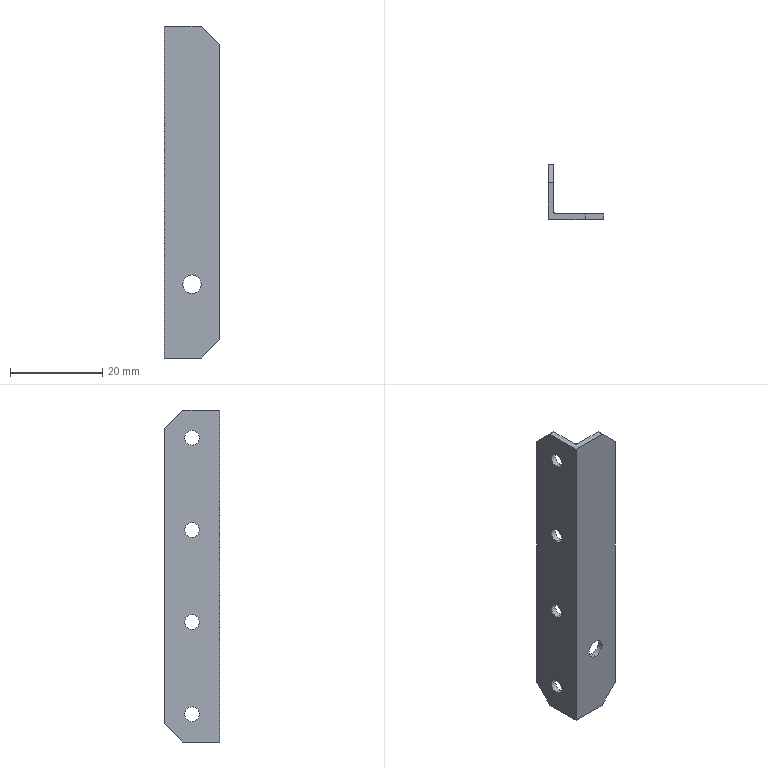Part | SolidWorks | features BaseBody 1 | 1 solid | 23 faces | box 12 x 12 x 72 mm | volume 1882 mm3 | plane 12 | cylinder 11 | commonest cylinder face diameters 3.2 x8 4 x2 1 x1
STEP:
#1=CARTESIAN_POINT('',(6.,0.,18.));
#2=VERTEX_POINT('',#1);
#3=CARTESIAN_POINT('',(6.,0.,14.));
#4=VERTEX_POINT('',#3);
#5=CARTESIAN_POINT('',(6.,0.,16.));
#6=DIRECTION('',(0.,-1.,0.));
#7=DIRECTION('',(0.,0.,1.));
#8=AXIS2_PLACEMENT_3D('',#5,#6,#7);
#9=CIRCLE('',#8,2.);
#10=EDGE_CURVE('',#2,#4,#9,.T.);
#11=ORIENTED_EDGE('',*,*,#10,.T.);
#12=CARTESIAN_POINT('',(6.,1.2,14.));
#13=VERTEX_POINT('',#12);
#14=CARTESIAN_POINT('',(6.,0.,14.));
#15=DIRECTION('',(0.,1.,0.));
#16=VECTOR('',#15,1000.);
#17=LINE('',#14,#16);
#18=EDGE_CURVE('',#4,#13,#17,.T.);
#19=ORIENTED_EDGE('',*,*,#18,.T.);
#20=CARTESIAN_POINT('',(6.,1.2,18.));
#21=VERTEX_POINT('',#20);
#22=CARTESIAN_POINT('',(6.,1.2,16.));
#23=DIRECTION('',(0.,1.,0.));
#24=DIRECTION('',(0.,0.,1.));
#25=AXIS2_PLACEMENT_3D('',#22,#23,#24);
#26=CIRCLE('',#25,2.);
#27=EDGE_CURVE('',#13,#21,#26,.T.);
#28=ORIENTED_EDGE('',*,*,#27,.T.);
#29=CARTESIAN_POINT('',(6.,0.,18.));
#30=DIRECTION('',(0.,1.,0.));
#31=VECTOR('',#30,1000.);
#32=LINE('',#29,#31);
#33=EDGE_CURVE('',#2,#21,#32,.T.);
#34=ORIENTED_EDGE('',*,*,#33,.F.);
#35=EDGE_LOOP('',(#11,#19,#28,#34));
#36=FACE_OUTER_BOUND('',#35,.T.);
#37=CARTESIAN_POINT('',(6.,0.,16.));
#38=DIRECTION('',(0.,1.,0.));
#39=DIRECTION('',(0.,0.,1.));
#40=AXIS2_PLACEMENT_3D('',#37,#38,#39);
#41=CYLINDRICAL_SURFACE('',#40,2.);
#42=ADVANCED_FACE('',(#36),#41,.F.);
#43=CARTESIAN_POINT('',(1.2,6.,7.6));
#44=VERTEX_POINT('',#43);
#45=CARTESIAN_POINT('',(1.2,6.,4.4));
#46=VERTEX_POINT('',#45);
#47=CARTESIAN_POINT('',(1.2,6.,6.));
#48=DIRECTION('',(1.,0.,0.));
#49=DIRECTION('',(0.,0.,1.));
#50=AXIS2_PLACEMENT_3D('',#47,#48,#49);
#51=CIRCLE('',#50,1.6);
#52=EDGE_CURVE('',#44,#46,#51,.T.);
#53=ORIENTED_EDGE('',*,*,#52,.T.);
#54=CARTESIAN_POINT('',(0.,6.,4.4));
#55=VERTEX_POINT('',#54);
#56=CARTESIAN_POINT('',(1.2,6.,4.4));
#57=DIRECTION('',(-1.,0.,0.));
#58=VECTOR('',#57,1000.);
#59=LINE('',#56,#58);
#60=EDGE_CURVE('',#46,#55,#59,.T.);
#61=ORIENTED_EDGE('',*,*,#60,.T.);
#62=CARTESIAN_POINT('',(0.,6.,7.6));
#63=VERTEX_POINT('',#62);
#64=CARTESIAN_POINT('',(0.,6.,6.));
#65=DIRECTION('',(-1.,0.,0.));
#66=DIRECTION('',(0.,0.,1.));
#67=AXIS2_PLACEMENT_3D('',#64,#65,#66);
#68=CIRCLE('',#67,1.6);
#69=EDGE_CURVE('',#55,#63,#68,.T.);
#70=ORIENTED_EDGE('',*,*,#69,.T.);
#71=CARTESIAN_POINT('',(1.2,6.,7.6));
#72=DIRECTION('',(-1.,0.,0.));
#73=VECTOR('',#72,1000.);
#74=LINE('',#71,#73);
#75=EDGE_CURVE('',#44,#63,#74,.T.);
#76=ORIENTED_EDGE('',*,*,#75,.F.);
#77=EDGE_LOOP('',(#53,#61,#70,#76));
#78=FACE_OUTER_BOUND('',#77,.T.);
#79=CARTESIAN_POINT('',(1.2,6.,6.));
#80=DIRECTION('',(-1.,0.,0.));
#81=DIRECTION('',(0.,0.,1.));
#82=AXIS2_PLACEMENT_3D('',#79,#80,#81);
#83=CYLINDRICAL_SURFACE('',#82,1.6);
#84=ADVANCED_FACE('',(#78),#83,.F.);
#85=CARTESIAN_POINT('',(1.2,6.,67.6));
#86=VERTEX_POINT('',#85);
#87=CARTESIAN_POINT('',(1.2,6.,64.4));
#88=VERTEX_POINT('',#87);
#89=CARTESIAN_POINT('',(1.2,6.,66.));
#90=DIRECTION('',(1.,0.,0.));
#91=DIRECTION('',(0.,0.,1.));
#92=AXIS2_PLACEMENT_3D('',#89,#90,#91);
#93=CIRCLE('',#92,1.6);
#94=EDGE_CURVE('',#86,#88,#93,.T.);
#95=ORIENTED_EDGE('',*,*,#94,.T.);
#96=CARTESIAN_POINT('',(0.,6.,64.4));
#97=VERTEX_POINT('',#96);
#98=CARTESIAN_POINT('',(1.2,6.,64.4));
#99=DIRECTION('',(-1.,0.,0.));
#100=VECTOR('',#99,1000.);
#101=LINE('',#98,#100);
#102=EDGE_CURVE('',#88,#97,#101,.T.);
#103=ORIENTED_EDGE('',*,*,#102,.T.);
#104=CARTESIAN_POINT('',(0.,6.,67.6));
#105=VERTEX_POINT('',#104);
#106=CARTESIAN_POINT('',(0.,6.,66.));
#107=DIRECTION('',(-1.,0.,0.));
#108=DIRECTION('',(0.,0.,1.));
#109=AXIS2_PLACEMENT_3D('',#106,#107,#108);
#110=CIRCLE('',#109,1.6);
#111=EDGE_CURVE('',#97,#105,#110,.T.);
#112=ORIENTED_EDGE('',*,*,#111,.T.);
#113=CARTESIAN_POINT('',(1.2,6.,67.6));
#114=DIRECTION('',(-1.,0.,0.));
#115=VECTOR('',#114,1000.);
#116=LINE('',#113,#115);
#117=EDGE_CURVE('',#86,#105,#116,.T.);
#118=ORIENTED_EDGE('',*,*,#117,.F.);
#119=EDGE_LOOP('',(#95,#103,#112,#118));
#120=FACE_OUTER_BOUND('',#119,.T.);
#121=CARTESIAN_POINT('',(1.2,6.,66.));
#122=DIRECTION('',(-1.,0.,0.));
#123=DIRECTION('',(0.,0.,1.));
#124=AXIS2_PLACEMENT_3D('',#121,#122,#123);
#125=CYLINDRICAL_SURFACE('',#124,1.6);
#126=ADVANCED_FACE('',(#120),#125,.F.);
#127=CARTESIAN_POINT('',(1.2,6.,27.6));
#128=VERTEX_POINT('',#127);
#129=CARTESIAN_POINT('',(1.2,6.,24.4));
#130=VERTEX_POINT('',#129);
#131=CARTESIAN_POINT('',(1.2,6.,26.));
#132=DIRECTION('',(1.,0.,0.));
#133=DIRECTION('',(0.,0.,1.));
#134=AXIS2_PLACEMENT_3D('',#131,#132,#133);
#135=CIRCLE('',#134,1.6);
#136=EDGE_CURVE('',#128,#130,#135,.T.);
#137=ORIENTED_EDGE('',*,*,#136,.T.);
#138=CARTESIAN_POINT('',(0.,6.,24.4));
#139=VERTEX_POINT('',#138);
#140=CARTESIAN_POINT('',(1.2,6.,24.4));
#141=DIRECTION('',(-1.,0.,0.));
#142=VECTOR('',#141,1000.);
#143=LINE('',#140,#142);
#144=EDGE_CURVE('',#130,#139,#143,.T.);
#145=ORIENTED_EDGE('',*,*,#144,.T.);
#146=CARTESIAN_POINT('',(0.,6.,27.6));
#147=VERTEX_POINT('',#146);
#148=CARTESIAN_POINT('',(0.,6.,26.));
#149=DIRECTION('',(-1.,0.,0.));
#150=DIRECTION('',(0.,0.,1.));
#151=AXIS2_PLACEMENT_3D('',#148,#149,#150);
#152=CIRCLE('',#151,1.6);
#153=EDGE_CURVE('',#139,#147,#152,.T.);
#154=ORIENTED_EDGE('',*,*,#153,.T.);
#155=CARTESIAN_POINT('',(1.2,6.,27.6));
#156=DIRECTION('',(-1.,0.,0.));
#157=VECTOR('',#156,1000.);
#158=LINE('',#155,#157);
#159=EDGE_CURVE('',#128,#147,#158,.T.);
#160=ORIENTED_EDGE('',*,*,#159,.F.);
#161=EDGE_LOOP('',(#137,#145,#154,#160));
#162=FACE_OUTER_BOUND('',#161,.T.);
#163=CARTESIAN_POINT('',(1.2,6.,26.));
#164=DIRECTION('',(-1.,0.,0.));
#165=DIRECTION('',(0.,0.,1.));
#166=AXIS2_PLACEMENT_3D('',#163,#164,#165);
#167=CYLINDRICAL_SURFACE('',#166,1.6);
#168=ADVANCED_FACE('',(#162),#167,.F.);
#169=CARTESIAN_POINT('',(1.2,6.,47.6));
#170=VERTEX_POINT('',#169);
#171=CARTESIAN_POINT('',(1.2,6.,44.4));
#172=VERTEX_POINT('',#171);
#173=CARTESIAN_POINT('',(1.2,6.,46.));
#174=DIRECTION('',(1.,0.,0.));
#175=DIRECTION('',(0.,0.,1.));
#176=AXIS2_PLACEMENT_3D('',#173,#174,#175);
#177=CIRCLE('',#176,1.6);
#178=EDGE_CURVE('',#170,#172,#177,.T.);
#179=ORIENTED_EDGE('',*,*,#178,.T.);
#180=CARTESIAN_POINT('',(0.,6.,44.4));
#181=VERTEX_POINT('',#180);
#182=CARTESIAN_POINT('',(1.2,6.,44.4));
#183=DIRECTION('',(-1.,0.,0.));
#184=VECTOR('',#183,1000.);
#185=LINE('',#182,#184);
#186=EDGE_CURVE('',#172,#181,#185,.T.);
#187=ORIENTED_EDGE('',*,*,#186,.T.);
#188=CARTESIAN_POINT('',(0.,6.,47.6));
#189=VERTEX_POINT('',#188);
#190=CARTESIAN_POINT('',(0.,6.,46.));
#191=DIRECTION('',(-1.,0.,0.));
#192=DIRECTION('',(0.,0.,1.));
#193=AXIS2_PLACEMENT_3D('',#190,#191,#192);
#194=CIRCLE('',#193,1.6);
#195=EDGE_CURVE('',#181,#189,#194,.T.);
#196=ORIENTED_EDGE('',*,*,#195,.T.);
#197=CARTESIAN_POINT('',(1.2,6.,47.6));
#198=DIRECTION('',(-1.,0.,0.));
#199=VECTOR('',#198,1000.);
#200=LINE('',#197,#199);
#201=EDGE_CURVE('',#170,#189,#200,.T.);
#202=ORIENTED_EDGE('',*,*,#201,.F.);
#203=EDGE_LOOP('',(#179,#187,#196,#202));
#204=FACE_OUTER_BOUND('',#203,.T.);
#205=CARTESIAN_POINT('',(1.2,6.,46.));
#206=DIRECTION('',(-1.,0.,0.));
#207=DIRECTION('',(0.,0.,1.));
#208=AXIS2_PLACEMENT_3D('',#205,#206,#207);
#209=CYLINDRICAL_SURFACE('',#208,1.6);
#210=ADVANCED_FACE('',(#204),#209,.F.);
#211=ORIENTED_EDGE('',*,*,#18,.F.);
#212=CARTESIAN_POINT('',(6.,0.,16.));
#213=DIRECTION('',(0.,-1.,0.));
#214=DIRECTION('',(0.,0.,1.));
#215=AXIS2_PLACEMENT_3D('',#212,#213,#214);
#216=CIRCLE('',#215,2.);
#217=EDGE_CURVE('',#4,#2,#216,.T.);
#218=ORIENTED_EDGE('',*,*,#217,.T.);
#219=ORIENTED_EDGE('',*,*,#33,.T.);
#220=CARTESIAN_POINT('',(6.,1.2,16.));
#221=DIRECTION('',(0.,1.,0.));
#222=DIRECTION('',(0.,0.,1.));
#223=AXIS2_PLACEMENT_3D('',#220,#221,#222);
#224=CIRCLE('',#223,2.);
#225=EDGE_CURVE('',#21,#13,#224,.T.);
#226=ORIENTED_EDGE('',*,*,#225,.T.);
#227=EDGE_LOOP('',(#211,#218,#219,#226));
#228=FACE_OUTER_BOUND('',#227,.T.);
#229=CARTESIAN_POINT('',(6.,0.,16.));
#230=DIRECTION('',(0.,1.,0.));
#231=DIRECTION('',(0.,0.,1.));
#232=AXIS2_PLACEMENT_3D('',#229,#230,#231);
#233=CYLINDRICAL_SURFACE('',#232,2.);
#234=ADVANCED_FACE('',(#228),#233,.F.);
#235=ORIENTED_EDGE('',*,*,#225,.F.);
#236=ORIENTED_EDGE('',*,*,#27,.F.);
#237=EDGE_LOOP('',(#235,#236));
#238=FACE_BOUND('',#237,.T.);
#239=CARTESIAN_POINT('',(8.,1.2,0.));
#240=VERTEX_POINT('',#239);
#241=CARTESIAN_POINT('',(12.,1.2,4.));
#242=VERTEX_POINT('',#241);
#243=CARTESIAN_POINT('',(8.,1.2,0.));
#244=DIRECTION('',(0.7071,0.,0.7071));
#245=VECTOR('',#244,1000.);
#246=LINE('',#243,#245);
#247=EDGE_CURVE('',#240,#242,#246,.T.);
#248=ORIENTED_EDGE('',*,*,#247,.F.);
#249=CARTESIAN_POINT('',(1.7,1.2,0.));
#250=VERTEX_POINT('',#249);
#251=CARTESIAN_POINT('',(6.85,1.2,0.));
#252=DIRECTION('',(1.,0.,0.));
#253=VECTOR('',#252,1000.);
#254=LINE('',#251,#253);
#255=EDGE_CURVE('',#250,#240,#254,.T.);
#256=ORIENTED_EDGE('',*,*,#255,.F.);
#257=CARTESIAN_POINT('',(1.7,1.2,72.));
#258=VERTEX_POINT('',#257);
#259=CARTESIAN_POINT('',(1.7,1.2,36.));
#260=DIRECTION('',(0.,0.,-1.));
#261=VECTOR('',#260,1000.);
#262=LINE('',#259,#261);
#263=EDGE_CURVE('',#258,#250,#262,.T.);
#264=ORIENTED_EDGE('',*,*,#263,.F.);
#265=CARTESIAN_POINT('',(8.,1.2,72.));
#266=VERTEX_POINT('',#265);
#267=CARTESIAN_POINT('',(6.85,1.2,72.));
#268=DIRECTION('',(-1.,0.,0.));
#269=VECTOR('',#268,1000.);
#270=LINE('',#267,#269);
#271=EDGE_CURVE('',#266,#258,#270,.T.);
#272=ORIENTED_EDGE('',*,*,#271,.F.);
#273=CARTESIAN_POINT('',(12.,1.2,68.));
#274=VERTEX_POINT('',#273);
#275=CARTESIAN_POINT('',(8.,1.2,72.));
#276=DIRECTION('',(-0.7071,0.,0.7071));
#277=VECTOR('',#276,1000.);
#278=LINE('',#275,#277);
#279=EDGE_CURVE('',#274,#266,#278,.T.);
#280=ORIENTED_EDGE('',*,*,#279,.F.);
#281=CARTESIAN_POINT('',(12.,1.2,36.));
#282=DIRECTION('',(0.,0.,1.));
#283=VECTOR('',#282,1000.);
#284=LINE('',#281,#283);
#285=EDGE_CURVE('',#242,#274,#284,.T.);
#286=ORIENTED_EDGE('',*,*,#285,.F.);
#287=EDGE_LOOP('',(#248,#256,#264,#272,#280,#286));
#288=FACE_OUTER_BOUND('',#287,.T.);
#289=CARTESIAN_POINT('',(1.7,1.2,72.));
#290=DIRECTION('',(0.,-1.,0.));
#291=DIRECTION('',(0.,0.,-1.));
#292=AXIS2_PLACEMENT_3D('',#289,#290,#291);
#293=PLANE('',#292);
#294=ADVANCED_FACE('',(#238,#288),#293,.F.);
#295=ORIENTED_EDGE('',*,*,#10,.F.);
#296=ORIENTED_EDGE('',*,*,#217,.F.);
#297=EDGE_LOOP('',(#295,#296));
#298=FACE_BOUND('',#297,.T.);
#299=CARTESIAN_POINT('',(12.,0.,4.));
#300=VERTEX_POINT('',#299);
#301=CARTESIAN_POINT('',(8.,0.,0.));
#302=VERTEX_POINT('',#301);
#303=CARTESIAN_POINT('',(8.,0.,0.));
#304=DIRECTION('',(-0.7071,0.,-0.7071));
#305=VECTOR('',#304,1000.);
#306=LINE('',#303,#305);
#307=EDGE_CURVE('',#300,#302,#306,.T.);
#308=ORIENTED_EDGE('',*,*,#307,.F.);
#309=CARTESIAN_POINT('',(12.,0.,68.));
#310=VERTEX_POINT('',#309);
#311=CARTESIAN_POINT('',(12.,0.,36.));
#312=DIRECTION('',(0.,0.,-1.));
#313=VECTOR('',#312,1000.);
#314=LINE('',#311,#313);
#315=EDGE_CURVE('',#310,#300,#314,.T.);
#316=ORIENTED_EDGE('',*,*,#315,.F.);
#317=CARTESIAN_POINT('',(8.,0.,72.));
#318=VERTEX_POINT('',#317);
#319=CARTESIAN_POINT('',(8.,0.,72.));
#320=DIRECTION('',(0.7071,0.,-0.7071));
#321=VECTOR('',#320,1000.);
#322=LINE('',#319,#321);
#323=EDGE_CURVE('',#318,#310,#322,.T.);
#324=ORIENTED_EDGE('',*,*,#323,.F.);
#325=CARTESIAN_POINT('',(0.,0.,72.));
#326=VERTEX_POINT('',#325);
#327=CARTESIAN_POINT('',(6.,0.,72.));
#328=DIRECTION('',(1.,0.,0.));
#329=VECTOR('',#328,1000.);
#330=LINE('',#327,#329);
#331=EDGE_CURVE('',#326,#318,#330,.T.);
#332=ORIENTED_EDGE('',*,*,#331,.F.);
#333=CARTESIAN_POINT('',(0.,0.,0.));
#334=VERTEX_POINT('',#333);
#335=CARTESIAN_POINT('',(0.,0.,36.));
#336=DIRECTION('',(0.,0.,1.));
#337=VECTOR('',#336,1000.);
#338=LINE('',#335,#337);
#339=EDGE_CURVE('',#334,#326,#338,.T.);
#340=ORIENTED_EDGE('',*,*,#339,.F.);
#341=CARTESIAN_POINT('',(6.,0.,0.));
#342=DIRECTION('',(-1.,0.,0.));
#343=VECTOR('',#342,1000.);
#344=LINE('',#341,#343);
#345=EDGE_CURVE('',#302,#334,#344,.T.);
#346=ORIENTED_EDGE('',*,*,#345,.F.);
#347=EDGE_LOOP('',(#308,#316,#324,#332,#340,#346));
#348=FACE_OUTER_BOUND('',#347,.T.);
#349=CARTESIAN_POINT('',(0.,0.,0.));
#350=DIRECTION('',(0.,1.,0.));
#351=DIRECTION('',(0.,0.,1.));
#352=AXIS2_PLACEMENT_3D('',#349,#350,#351);
#353=PLANE('',#352);
#354=ADVANCED_FACE('',(#298,#348),#353,.F.);
#355=CARTESIAN_POINT('',(12.,0.6,4.));
#356=DIRECTION('',(0.,-1.,0.));
#357=VECTOR('',#356,1000.);
#358=LINE('',#355,#357);
#359=EDGE_CURVE('',#242,#300,#358,.T.);
#360=ORIENTED_EDGE('',*,*,#359,.F.);
#361=ORIENTED_EDGE('',*,*,#285,.T.);
#362=CARTESIAN_POINT('',(12.,0.6,68.));
#363=DIRECTION('',(0.,1.,0.));
#364=VECTOR('',#363,1000.);
#365=LINE('',#362,#364);
#366=EDGE_CURVE('',#310,#274,#365,.T.);
#367=ORIENTED_EDGE('',*,*,#366,.F.);
#368=ORIENTED_EDGE('',*,*,#315,.T.);
#369=EDGE_LOOP('',(#360,#361,#367,#368));
#370=FACE_OUTER_BOUND('',#369,.T.);
#371=CARTESIAN_POINT('',(12.,0.,4.));
#372=DIRECTION('',(-1.,0.,0.));
#373=DIRECTION('',(0.,0.,1.));
#374=AXIS2_PLACEMENT_3D('',#371,#372,#373);
#375=PLANE('',#374);
#376=ADVANCED_FACE('',(#370),#375,.F.);
#377=CARTESIAN_POINT('',(8.,0.6,0.));
#378=DIRECTION('',(0.,-1.,0.));
#379=VECTOR('',#378,1000.);
#380=LINE('',#377,#379);
#381=EDGE_CURVE('',#240,#302,#380,.T.);
#382=ORIENTED_EDGE('',*,*,#381,.F.);
#383=ORIENTED_EDGE('',*,*,#247,.T.);
#384=ORIENTED_EDGE('',*,*,#359,.T.);
#385=ORIENTED_EDGE('',*,*,#307,.T.);
#386=EDGE_LOOP('',(#382,#383,#384,#385));
#387=FACE_OUTER_BOUND('',#386,.T.);
#388=CARTESIAN_POINT('',(8.,0.,0.));
#389=DIRECTION('',(-0.7071,0.,0.7071));
#390=DIRECTION('',(0.7071,0.,0.7071));
#391=AXIS2_PLACEMENT_3D('',#388,#389,#390);
#392=PLANE('',#391);
#393=ADVANCED_FACE('',(#387),#392,.F.);
#394=ORIENTED_EDGE('',*,*,#381,.T.);
#395=ORIENTED_EDGE('',*,*,#345,.T.);
#396=CARTESIAN_POINT('',(0.,8.,0.));
#397=VERTEX_POINT('',#396);
#398=CARTESIAN_POINT('',(0.,4.,0.));
#399=DIRECTION('',(0.,-1.,0.));
#400=VECTOR('',#399,1000.);
#401=LINE('',#398,#400);
#402=EDGE_CURVE('',#397,#334,#401,.T.);
#403=ORIENTED_EDGE('',*,*,#402,.F.);
#404=CARTESIAN_POINT('',(1.2,8.,0.));
#405=VERTEX_POINT('',#404);
#406=CARTESIAN_POINT('',(0.6,8.,0.));
#407=DIRECTION('',(1.,0.,0.));
#408=VECTOR('',#407,1000.);
#409=LINE('',#406,#408);
#410=EDGE_CURVE('',#397,#405,#409,.T.);
#411=ORIENTED_EDGE('',*,*,#410,.T.);
#412=CARTESIAN_POINT('',(1.2,1.7,0.));
#413=VERTEX_POINT('',#412);
#414=CARTESIAN_POINT('',(1.2,4.,0.));
#415=DIRECTION('',(0.,1.,0.));
#416=VECTOR('',#415,1000.);
#417=LINE('',#414,#416);
#418=EDGE_CURVE('',#413,#405,#417,.T.);
#419=ORIENTED_EDGE('',*,*,#418,.F.);
#420=CARTESIAN_POINT('',(1.7,1.7,0.));
#421=DIRECTION('',(0.,0.,-1.));
#422=DIRECTION('',(-1.,0.,0.));
#423=AXIS2_PLACEMENT_3D('',#420,#421,#422);
#424=CIRCLE('',#423,0.5);
#425=EDGE_CURVE('',#250,#413,#424,.T.);
#426=ORIENTED_EDGE('',*,*,#425,.F.);
#427=ORIENTED_EDGE('',*,*,#255,.T.);
#428=EDGE_LOOP('',(#394,#395,#403,#411,#419,#426,#427));
#429=FACE_OUTER_BOUND('',#428,.T.);
#430=CARTESIAN_POINT('',(0.,0.,0.));
#431=DIRECTION('',(0.,0.,1.));
#432=DIRECTION('',(1.,0.,0.));
#433=AXIS2_PLACEMENT_3D('',#430,#431,#432);
#434=PLANE('',#433);
#435=ADVANCED_FACE('',(#429),#434,.F.);
#436=CARTESIAN_POINT('',(1.2,1.7,72.));
#437=VERTEX_POINT('',#436);
#438=CARTESIAN_POINT('',(1.7,1.7,72.));
#439=DIRECTION('',(0.,0.,1.));
#440=DIRECTION('',(-1.,0.,0.));
#441=AXIS2_PLACEMENT_3D('',#438,#439,#440);
#442=CIRCLE('',#441,0.5);
#443=EDGE_CURVE('',#437,#258,#442,.T.);
#444=ORIENTED_EDGE('',*,*,#443,.T.);
#445=ORIENTED_EDGE('',*,*,#263,.T.);
#446=ORIENTED_EDGE('',*,*,#425,.T.);
#447=CARTESIAN_POINT('',(1.2,1.7,36.));
#448=DIRECTION('',(0.,0.,1.));
#449=VECTOR('',#448,1000.);
#450=LINE('',#447,#449);
#451=EDGE_CURVE('',#413,#437,#450,.T.);
#452=ORIENTED_EDGE('',*,*,#451,.T.);
#453=EDGE_LOOP('',(#444,#445,#446,#452));
#454=FACE_OUTER_BOUND('',#453,.T.);
#455=CARTESIAN_POINT('',(1.7,1.7,72.));
#456=DIRECTION('',(0.,0.,-1.));
#457=DIRECTION('',(-1.,0.,0.));
#458=AXIS2_PLACEMENT_3D('',#455,#456,#457);
#459=CYLINDRICAL_SURFACE('',#458,0.5);
#460=ADVANCED_FACE('',(#454),#459,.F.);
#461=CARTESIAN_POINT('',(0.,8.,72.));
#462=VERTEX_POINT('',#461);
#463=CARTESIAN_POINT('',(1.2,8.,72.));
#464=VERTEX_POINT('',#463);
#465=CARTESIAN_POINT('',(0.6,8.,72.));
#466=DIRECTION('',(1.,0.,0.));
#467=VECTOR('',#466,1000.);
#468=LINE('',#465,#467);
#469=EDGE_CURVE('',#462,#464,#468,.T.);
#470=ORIENTED_EDGE('',*,*,#469,.F.);
#471=CARTESIAN_POINT('',(0.,4.,72.));
#472=DIRECTION('',(0.,-1.,0.));
#473=VECTOR('',#472,1000.);
#474=LINE('',#471,#473);
#475=EDGE_CURVE('',#462,#326,#474,.T.);
#476=ORIENTED_EDGE('',*,*,#475,.T.);
#477=ORIENTED_EDGE('',*,*,#331,.T.);
#478=CARTESIAN_POINT('',(8.,4.,72.));
#479=DIRECTION('',(0.,1.,0.));
#480=VECTOR('',#479,1000.);
#481=LINE('',#478,#480);
#482=EDGE_CURVE('',#318,#266,#481,.T.);
#483=ORIENTED_EDGE('',*,*,#482,.T.);
#484=ORIENTED_EDGE('',*,*,#271,.T.);
#485=ORIENTED_EDGE('',*,*,#443,.F.);
#486=CARTESIAN_POINT('',(1.2,4.,72.));
#487=DIRECTION('',(0.,1.,0.));
#488=VECTOR('',#487,1000.);
#489=LINE('',#486,#488);
#490=EDGE_CURVE('',#437,#464,#489,.T.);
#491=ORIENTED_EDGE('',*,*,#490,.T.);
#492=EDGE_LOOP('',(#470,#476,#477,#483,#484,#485,#491));
#493=FACE_OUTER_BOUND('',#492,.T.);
#494=CARTESIAN_POINT('',(0.,0.,72.));
#495=DIRECTION('',(0.,0.,1.));
#496=DIRECTION('',(1.,0.,0.));
#497=AXIS2_PLACEMENT_3D('',#494,#495,#496);
#498=PLANE('',#497);
#499=ADVANCED_FACE('',(#493),#498,.T.);
#500=ORIENTED_EDGE('',*,*,#279,.T.);
#501=ORIENTED_EDGE('',*,*,#482,.F.);
#502=ORIENTED_EDGE('',*,*,#323,.T.);
#503=ORIENTED_EDGE('',*,*,#366,.T.);
#504=EDGE_LOOP('',(#500,#501,#502,#503));
#505=FACE_OUTER_BOUND('',#504,.T.);
#506=CARTESIAN_POINT('',(8.,0.,72.));
#507=DIRECTION('',(0.7071,0.,0.7071));
#508=DIRECTION('',(0.7071,0.,-0.7071));
#509=AXIS2_PLACEMENT_3D('',#506,#507,#508);
#510=PLANE('',#509);
#511=ADVANCED_FACE('',(#505),#510,.T.);
#512=CARTESIAN_POINT('',(0.,6.,6.));
#513=DIRECTION('',(-1.,0.,0.));
#514=DIRECTION('',(0.,0.,1.));
#515=AXIS2_PLACEMENT_3D('',#512,#513,#514);
#516=CIRCLE('',#515,1.6);
#517=EDGE_CURVE('',#63,#55,#516,.T.);
#518=ORIENTED_EDGE('',*,*,#517,.F.);
#519=ORIENTED_EDGE('',*,*,#69,.F.);
#520=EDGE_LOOP('',(#518,#519));
#521=FACE_BOUND('',#520,.T.);
#522=CARTESIAN_POINT('',(0.,6.,66.));
#523=DIRECTION('',(-1.,0.,0.));
#524=DIRECTION('',(0.,0.,1.));
#525=AXIS2_PLACEMENT_3D('',#522,#523,#524);
#526=CIRCLE('',#525,1.6);
#527=EDGE_CURVE('',#105,#97,#526,.T.);
#528=ORIENTED_EDGE('',*,*,#527,.F.);
#529=ORIENTED_EDGE('',*,*,#111,.F.);
#530=EDGE_LOOP('',(#528,#529));
#531=FACE_BOUND('',#530,.T.);
#532=CARTESIAN_POINT('',(0.,6.,26.));
#533=DIRECTION('',(-1.,0.,0.));
#534=DIRECTION('',(0.,0.,1.));
#535=AXIS2_PLACEMENT_3D('',#532,#533,#534);
#536=CIRCLE('',#535,1.6);
#537=EDGE_CURVE('',#147,#139,#536,.T.);
#538=ORIENTED_EDGE('',*,*,#537,.F.);
#539=ORIENTED_EDGE('',*,*,#153,.F.);
#540=EDGE_LOOP('',(#538,#539));
#541=FACE_BOUND('',#540,.T.);
#542=CARTESIAN_POINT('',(0.,6.,46.));
#543=DIRECTION('',(-1.,0.,0.));
#544=DIRECTION('',(0.,0.,1.));
#545=AXIS2_PLACEMENT_3D('',#542,#543,#544);
#546=CIRCLE('',#545,1.6);
#547=EDGE_CURVE('',#189,#181,#546,.T.);
#548=ORIENTED_EDGE('',*,*,#547,.F.);
#549=ORIENTED_EDGE('',*,*,#195,.F.);
#550=EDGE_LOOP('',(#548,#549));
#551=FACE_BOUND('',#550,.T.);
#552=CARTESIAN_POINT('',(0.,12.,4.));
#553=VERTEX_POINT('',#552);
#554=CARTESIAN_POINT('',(0.,12.,4.));
#555=DIRECTION('',(0.,0.7071,0.7071));
#556=VECTOR('',#555,1000.);
#557=LINE('',#554,#556);
#558=EDGE_CURVE('',#397,#553,#557,.T.);
#559=ORIENTED_EDGE('',*,*,#558,.F.);
#560=ORIENTED_EDGE('',*,*,#402,.T.);
#561=ORIENTED_EDGE('',*,*,#339,.T.);
#562=ORIENTED_EDGE('',*,*,#475,.F.);
#563=CARTESIAN_POINT('',(0.,12.,68.));
#564=VERTEX_POINT('',#563);
#565=CARTESIAN_POINT('',(0.,12.,68.));
#566=DIRECTION('',(0.,-0.7071,0.7071));
#567=VECTOR('',#566,1000.);
#568=LINE('',#565,#567);
#569=EDGE_CURVE('',#564,#462,#568,.T.);
#570=ORIENTED_EDGE('',*,*,#569,.F.);
#571=CARTESIAN_POINT('',(0.,12.,36.));
#572=DIRECTION('',(0.,0.,1.));
#573=VECTOR('',#572,1000.);
#574=LINE('',#571,#573);
#575=EDGE_CURVE('',#553,#564,#574,.T.);
#576=ORIENTED_EDGE('',*,*,#575,.F.);
#577=EDGE_LOOP('',(#559,#560,#561,#562,#570,#576));
#578=FACE_OUTER_BOUND('',#577,.T.);
#579=CARTESIAN_POINT('',(0.,0.,0.));
#580=DIRECTION('',(1.,0.,0.));
#581=DIRECTION('',(0.,1.,0.));
#582=AXIS2_PLACEMENT_3D('',#579,#580,#581);
#583=PLANE('',#582);
#584=ADVANCED_FACE('',(#521,#531,#541,#551,#578),#583,.F.);
#585=ORIENTED_EDGE('',*,*,#52,.F.);
#586=CARTESIAN_POINT('',(1.2,6.,6.));
#587=DIRECTION('',(1.,0.,0.));
#588=DIRECTION('',(0.,0.,1.));
#589=AXIS2_PLACEMENT_3D('',#586,#587,#588);
#590=CIRCLE('',#589,1.6);
#591=EDGE_CURVE('',#46,#44,#590,.T.);
#592=ORIENTED_EDGE('',*,*,#591,.F.);
#593=EDGE_LOOP('',(#585,#592));
#594=FACE_BOUND('',#593,.T.);
#595=ORIENTED_EDGE('',*,*,#94,.F.);
#596=CARTESIAN_POINT('',(1.2,6.,66.));
#597=DIRECTION('',(1.,0.,0.));
#598=DIRECTION('',(0.,0.,1.));
#599=AXIS2_PLACEMENT_3D('',#596,#597,#598);
#600=CIRCLE('',#599,1.6);
#601=EDGE_CURVE('',#88,#86,#600,.T.);
#602=ORIENTED_EDGE('',*,*,#601,.F.);
#603=EDGE_LOOP('',(#595,#602));
#604=FACE_BOUND('',#603,.T.);
#605=ORIENTED_EDGE('',*,*,#136,.F.);
#606=CARTESIAN_POINT('',(1.2,6.,26.));
#607=DIRECTION('',(1.,0.,0.));
#608=DIRECTION('',(0.,0.,1.));
#609=AXIS2_PLACEMENT_3D('',#606,#607,#608);
#610=CIRCLE('',#609,1.6);
#611=EDGE_CURVE('',#130,#128,#610,.T.);
#612=ORIENTED_EDGE('',*,*,#611,.F.);
#613=EDGE_LOOP('',(#605,#612));
#614=FACE_BOUND('',#613,.T.);
#615=ORIENTED_EDGE('',*,*,#178,.F.);
#616=CARTESIAN_POINT('',(1.2,6.,46.));
#617=DIRECTION('',(1.,0.,0.));
#618=DIRECTION('',(0.,0.,1.));
#619=AXIS2_PLACEMENT_3D('',#616,#617,#618);
#620=CIRCLE('',#619,1.6);
#621=EDGE_CURVE('',#172,#170,#620,.T.);
#622=ORIENTED_EDGE('',*,*,#621,.F.);
#623=EDGE_LOOP('',(#615,#622));
#624=FACE_BOUND('',#623,.T.);
#625=CARTESIAN_POINT('',(1.2,12.,4.));
#626=VERTEX_POINT('',#625);
#627=CARTESIAN_POINT('',(1.2,12.,4.));
#628=DIRECTION('',(0.,-0.7071,-0.7071));
#629=VECTOR('',#628,1000.);
#630=LINE('',#627,#629);
#631=EDGE_CURVE('',#626,#405,#630,.T.);
#632=ORIENTED_EDGE('',*,*,#631,.F.);
#633=CARTESIAN_POINT('',(1.2,12.,68.));
#634=VERTEX_POINT('',#633);
#635=CARTESIAN_POINT('',(1.2,12.,36.));
#636=DIRECTION('',(0.,0.,-1.));
#637=VECTOR('',#636,1000.);
#638=LINE('',#635,#637);
#639=EDGE_CURVE('',#634,#626,#638,.T.);
#640=ORIENTED_EDGE('',*,*,#639,.F.);
#641=CARTESIAN_POINT('',(1.2,12.,68.));
#642=DIRECTION('',(0.,0.7071,-0.7071));
#643=VECTOR('',#642,1000.);
#644=LINE('',#641,#643);
#645=EDGE_CURVE('',#464,#634,#644,.T.);
#646=ORIENTED_EDGE('',*,*,#645,.F.);
#647=ORIENTED_EDGE('',*,*,#490,.F.);
#648=ORIENTED_EDGE('',*,*,#451,.F.);
#649=ORIENTED_EDGE('',*,*,#418,.T.);
#650=EDGE_LOOP('',(#632,#640,#646,#647,#648,#649));
#651=FACE_OUTER_BOUND('',#650,.T.);
#652=CARTESIAN_POINT('',(1.2,1.7,0.));
#653=DIRECTION('',(-1.,0.,0.));
#654=DIRECTION('',(0.,0.,1.));
#655=AXIS2_PLACEMENT_3D('',#652,#653,#654);
#656=PLANE('',#655);
#657=ADVANCED_FACE('',(#594,#604,#614,#624,#651),#656,.F.);
#658=ORIENTED_EDGE('',*,*,#60,.F.);
#659=ORIENTED_EDGE('',*,*,#591,.T.);
#660=ORIENTED_EDGE('',*,*,#75,.T.);
#661=ORIENTED_EDGE('',*,*,#517,.T.);
#662=EDGE_LOOP('',(#658,#659,#660,#661));
#663=FACE_OUTER_BOUND('',#662,.T.);
#664=CARTESIAN_POINT('',(1.2,6.,6.));
#665=DIRECTION('',(-1.,0.,0.));
#666=DIRECTION('',(0.,0.,1.));
#667=AXIS2_PLACEMENT_3D('',#664,#665,#666);
#668=CYLINDRICAL_SURFACE('',#667,1.6);
#669=ADVANCED_FACE('',(#663),#668,.F.);
#670=ORIENTED_EDGE('',*,*,#102,.F.);
#671=ORIENTED_EDGE('',*,*,#601,.T.);
#672=ORIENTED_EDGE('',*,*,#117,.T.);
#673=ORIENTED_EDGE('',*,*,#527,.T.);
#674=EDGE_LOOP('',(#670,#671,#672,#673));
#675=FACE_OUTER_BOUND('',#674,.T.);
#676=CARTESIAN_POINT('',(1.2,6.,66.));
#677=DIRECTION('',(-1.,0.,0.));
#678=DIRECTION('',(0.,0.,1.));
#679=AXIS2_PLACEMENT_3D('',#676,#677,#678);
#680=CYLINDRICAL_SURFACE('',#679,1.6);
#681=ADVANCED_FACE('',(#675),#680,.F.);
#682=ORIENTED_EDGE('',*,*,#144,.F.);
#683=ORIENTED_EDGE('',*,*,#611,.T.);
#684=ORIENTED_EDGE('',*,*,#159,.T.);
#685=ORIENTED_EDGE('',*,*,#537,.T.);
#686=EDGE_LOOP('',(#682,#683,#684,#685));
#687=FACE_OUTER_BOUND('',#686,.T.);
#688=CARTESIAN_POINT('',(1.2,6.,26.));
#689=DIRECTION('',(-1.,0.,0.));
#690=DIRECTION('',(0.,0.,1.));
#691=AXIS2_PLACEMENT_3D('',#688,#689,#690);
#692=CYLINDRICAL_SURFACE('',#691,1.6);
#693=ADVANCED_FACE('',(#687),#692,.F.);
#694=ORIENTED_EDGE('',*,*,#186,.F.);
#695=ORIENTED_EDGE('',*,*,#621,.T.);
#696=ORIENTED_EDGE('',*,*,#201,.T.);
#697=ORIENTED_EDGE('',*,*,#547,.T.);
#698=EDGE_LOOP('',(#694,#695,#696,#697));
#699=FACE_OUTER_BOUND('',#698,.T.);
#700=CARTESIAN_POINT('',(1.2,6.,46.));
#701=DIRECTION('',(-1.,0.,0.));
#702=DIRECTION('',(0.,0.,1.));
#703=AXIS2_PLACEMENT_3D('',#700,#701,#702);
#704=CYLINDRICAL_SURFACE('',#703,1.6);
#705=ADVANCED_FACE('',(#699),#704,.F.);
#706=CARTESIAN_POINT('',(0.6,12.,4.));
#707=DIRECTION('',(1.,0.,0.));
#708=VECTOR('',#707,1000.);
#709=LINE('',#706,#708);
#710=EDGE_CURVE('',#553,#626,#709,.T.);
#711=ORIENTED_EDGE('',*,*,#710,.F.);
#712=ORIENTED_EDGE('',*,*,#575,.T.);
#713=CARTESIAN_POINT('',(0.6,12.,68.));
#714=DIRECTION('',(-1.,0.,0.));
#715=VECTOR('',#714,1000.);
#716=LINE('',#713,#715);
#717=EDGE_CURVE('',#634,#564,#716,.T.);
#718=ORIENTED_EDGE('',*,*,#717,.F.);
#719=ORIENTED_EDGE('',*,*,#639,.T.);
#720=EDGE_LOOP('',(#711,#712,#718,#719));
#721=FACE_OUTER_BOUND('',#720,.T.);
#722=CARTESIAN_POINT('',(0.,12.,68.));
#723=DIRECTION('',(0.,-1.,0.));
#724=DIRECTION('',(0.,0.,-1.));
#725=AXIS2_PLACEMENT_3D('',#722,#723,#724);
#726=PLANE('',#725);
#727=ADVANCED_FACE('',(#721),#726,.F.);
#728=ORIENTED_EDGE('',*,*,#410,.F.);
#729=ORIENTED_EDGE('',*,*,#558,.T.);
#730=ORIENTED_EDGE('',*,*,#710,.T.);
#731=ORIENTED_EDGE('',*,*,#631,.T.);
#732=EDGE_LOOP('',(#728,#729,#730,#731));
#733=FACE_OUTER_BOUND('',#732,.T.);
#734=CARTESIAN_POINT('',(0.,12.,4.));
#735=DIRECTION('',(0.,-0.7071,0.7071));
#736=DIRECTION('',(0.,-0.7071,-0.7071));
#737=AXIS2_PLACEMENT_3D('',#734,#735,#736);
#738=PLANE('',#737);
#739=ADVANCED_FACE('',(#733),#738,.F.);
#740=ORIENTED_EDGE('',*,*,#569,.T.);
#741=ORIENTED_EDGE('',*,*,#469,.T.);
#742=ORIENTED_EDGE('',*,*,#645,.T.);
#743=ORIENTED_EDGE('',*,*,#717,.T.);
#744=EDGE_LOOP('',(#740,#741,#742,#743));
#745=FACE_OUTER_BOUND('',#744,.T.);
#746=CARTESIAN_POINT('',(0.,12.,68.));
#747=DIRECTION('',(0.,0.7071,0.7071));
#748=DIRECTION('',(0.,-0.7071,0.7071));
#749=AXIS2_PLACEMENT_3D('',#746,#747,#748);
#750=PLANE('',#749);
#751=ADVANCED_FACE('',(#745),#750,.T.);
#752=CLOSED_SHELL('',(#42,#84,#126,#168,#210,#234,#294,#354,#376,#393,#435,#460,#499,#511,#584,#657,#669,#681,#693,#705,#727,#739,#751));
#753=MANIFOLD_SOLID_BREP('',#752);
#754=CARTESIAN_POINT('',(0.,0.,0.));
#755=DIRECTION('',(0.,0.,1.));
#756=DIRECTION('',(1.,0.,0.));
#757=AXIS2_PLACEMENT_3D('',#754,#755,#756);
#758=(LENGTH_UNIT()NAMED_UNIT(*)SI_UNIT(.MILLI.,.METRE.));
#759=UNCERTAINTY_MEASURE_WITH_UNIT(LENGTH_MEASURE(0.00001),#758,'','');
#760=(NAMED_UNIT(*)PLANE_ANGLE_UNIT()SI_UNIT($,.RADIAN.));
#761=(NAMED_UNIT(*)SI_UNIT($,.STERADIAN.)SOLID_ANGLE_UNIT());
#762=(GEOMETRIC_REPRESENTATION_CONTEXT(3)GLOBAL_UNCERTAINTY_ASSIGNED_CONTEXT((#759))GLOBAL_UNIT_ASSIGNED_CONTEXT((#758,#760,#761))REPRESENTATION_CONTEXT('',''));
#763=ADVANCED_BREP_SHAPE_REPRESENTATION('',(#753,#757),#762);